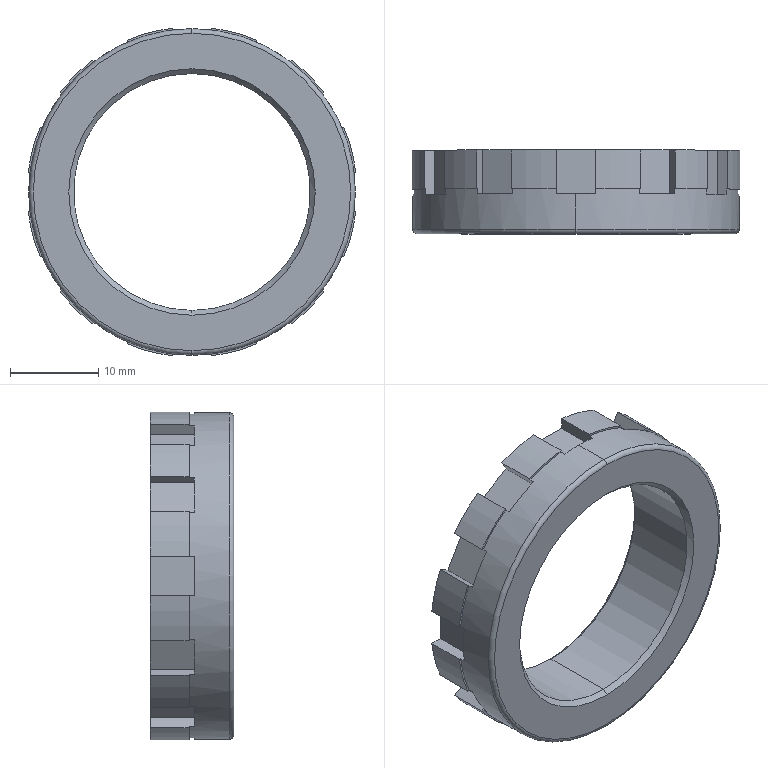Part | STEP file | AR20P-260S(20)_SETNUT_HI | 1 solid | 84 faces | box 37.229 x 9.5 x 37.229 mm | volume 4541 mm3 | plane 62 | cylinder 16 | cone 4 | torus 2 | commonest cylinder face diameters 37.5 x12 26.917 x2 37.07 x2